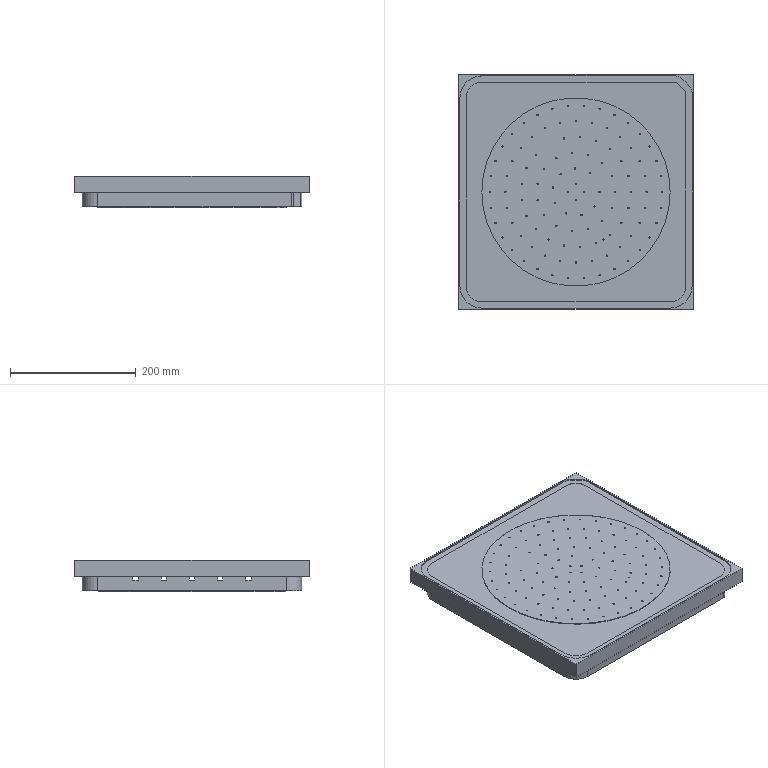NC program | NX | posted with a generic post | part box 374 x 374 x 49.5 mm
Lines 1 to 1179 of 17720:
N10 G17 G21 G94 G90
(01 , TOOL : D16R0.8)
N12 T00 M6
N14 G53
N16 G17 G0 G90 X-176.97 Y-25.521 S7000 M3 M8
N18 G43 Z105.5 H0
N20 Z26.5
N22 G94 G1 Y0. Z25.163 F4500.
N24 Y150.
N26 G2 X-150. Y176.97 R26.97
N28 G1 X157.929
N30 G2 X162.858 Y174.929 R6.97
N32 G1 X174.929 Y162.858
N34 G2 X176.97 Y157.929 R6.97
N36 G1 Y-150.
N38 G2 X150. Y-176.97 R26.97
N40 G1 X-150.
N42 G2 X-176.97 Y-150. R26.97
N44 G1 Y0.
N46 X-166.89
N48 Y150.
N50 G2 X-150. Y166.89 R16.89
N52 G1 X156.641
N54 X166.89 Y156.641
N56 Y-150.
N58 G2 X150. Y-166.89 R16.89
N60 G1 X-150.
N62 G2 X-166.89 Y-150. R16.89
N64 G1 Y0.
N66 X-156.81
N68 Y150.
N70 G2 X-150. Y156.81 R6.81
N72 G1 X152.466
N74 X156.81 Y152.466
N76 Y-150.
N78 G2 X150. Y-156.81 R6.81
N80 G1 X-150.
N82 G2 X-156.81 Y-150. R6.81
N84 G1 Y0.
N86 X-146.73
N88 Y146.73
N90 X146.73
N92 Y-146.73
N94 X-146.73
N96 Y0.
N98 X-136.65
N100 Y136.65
N102 X136.65
N104 Y-136.65
N106 X-136.65
N108 Y0.
N110 X-126.57
N112 Y126.57
N114 X126.57
N116 Y-126.57
N118 X-126.57
N120 Y0.
N122 X-116.49
N124 Y116.49
N126 X116.49
N128 Y-116.49
N130 X-116.49
N132 Y0.
N134 X-106.41
N136 Y106.41
N138 X106.41
N140 Y-106.41
N142 X-106.41
N144 Y0.
N146 X-96.33
N148 Y96.33
N150 X96.33
N152 Y-96.33
N154 X-96.33
N156 Y0.
N158 X-86.25
N160 Y86.25
N162 X86.25
N164 Y-86.25
N166 X-86.25
N168 Y0.
N170 X-76.17
N172 Y76.17
N174 X76.17
N176 Y-76.17
N178 X-76.17
N180 Y0.
N182 X-66.09
N184 Y66.09
N186 X66.09
N188 Y-66.09
N190 X-66.09
N192 Y0.
N194 X-56.01
N196 Y56.01
N198 X56.01
N200 Y-56.01
N202 X-56.01
N204 Y0.
N206 X-45.93
N208 Y45.93
N210 X45.93
N212 Y-45.93
N214 X-45.93
N216 Y0.
N218 X-35.85
N220 Y35.85
N222 X35.85
N224 Y-35.85
N226 X-35.85
N228 Y0.
N230 X-25.77
N232 Y25.77
N234 X25.77
N236 Y-25.77
N238 X-25.77
N240 Y0.
N242 X-15.69
N244 Y15.69
N246 X15.69
N248 Y-15.69
N250 X-15.69
N252 Y0.
N254 X-5.61
N256 Y5.61
N258 X5.61
N260 Y-5.61
N262 X-5.61
N264 Y0.
N266 G3 X-8.81 Y3.2 R3.2
N268 G1 Z26.163
N270 G0 Z28.5
N272 X-176.858 Y-25.521
N274 Z26.163
N276 G1 Y0. Z24.825
N278 Y150.
N280 G2 X-150. Y176.858 R26.858
N282 G1 X157.929
N284 G2 X162.778 Y174.85 R6.858
N286 G1 X174.85 Y162.778
N288 G2 X176.858 Y157.929 R6.858
N290 G1 Y-150.
N292 G2 X150. Y-176.858 R26.858
N294 G1 X-150.
N296 G2 X-176.858 Y-150. R26.858
N298 G1 Y0.
N300 X-166.778
N302 Y150.
N304 G2 X-150. Y166.778 R16.778
N306 G1 X156.594
N308 X166.778 Y156.594
N310 Y-150.
N312 G2 X150. Y-166.778 R16.778
N314 G1 X-150.
N316 G2 X-166.778 Y-150. R16.778
N318 G1 Y0.
N320 X-156.698
N322 Y150.
N324 G2 X-150. Y156.698 R6.698
N326 G1 X152.419
N328 X156.698 Y152.419
N330 Y-150.
N332 G2 X150. Y-156.698 R6.698
N334 G1 X-150.
N336 G2 X-156.698 Y-150. R6.698
N338 G1 Y0.
N340 X-146.618
N342 Y146.618
N344 X146.618
N346 Y-146.618
N348 X-146.618
N350 Y0.
N352 X-136.538
N354 Y136.538
N356 X136.538
N358 Y-136.538
N360 X-136.538
N362 Y0.
N364 X-126.458
N366 Y126.458
N368 X126.458
N370 Y-126.458
N372 X-126.458
N374 Y0.
N376 X-116.378
N378 Y116.378
N380 X116.378
N382 Y-116.378
N384 X-116.378
N386 Y0.
N388 X-106.298
N390 Y106.298
N392 X106.298
N394 Y-106.298
N396 X-106.298
N398 Y0.
N400 X-96.218
N402 Y96.218
N404 X96.218
N406 Y-96.218
N408 X-96.218
N410 Y0.
N412 X-86.138
N414 Y86.138
N416 X86.138
N418 Y-86.138
N420 X-86.138
N422 Y0.
N424 X-76.058
N426 Y76.058
N428 X76.058
N430 Y-76.058
N432 X-76.058
N434 Y0.
N436 X-65.978
N438 Y65.978
N440 X65.978
N442 Y-65.978
N444 X-65.978
N446 Y0.
N448 X-55.898
N450 Y55.898
N452 X55.898
N454 Y-55.898
N456 X-55.898
N458 Y0.
N460 X-45.818
N462 Y45.818
N464 X45.818
N466 Y-45.818
N468 X-45.818
N470 Y0.
N472 X-35.738
N474 Y35.738
N476 X35.738
N478 Y-35.738
N480 X-35.738
N482 Y0.
N484 X-25.658
N486 Y25.658
N488 X25.658
N490 Y-25.658
N492 X-25.658
N494 Y0.
N496 X-15.578
N498 Y15.578
N500 X15.578
N502 Y-15.578
N504 X-15.578
N506 Y0.
N508 X-5.498
N510 Y5.498
N512 X5.498
N514 Y-5.498
N516 X-5.498
N518 Y0.
N520 G3 X-8.698 Y3.2 R3.2
N522 G1 Z25.825
N524 G0 Z28.163
N526 X-176.85 Y-25.521
N528 Z25.825
N530 G1 Y0. Z24.488
N532 Y150.
N534 G2 X-150. Y176.85 R26.85
N536 G1 X157.929
N538 G2 X162.773 Y174.844 R6.85
N540 G1 X174.844 Y162.773
N542 G2 X176.85 Y157.929 R6.85
N544 G1 Y-150.
N546 G2 X150. Y-176.85 R26.85
N548 G1 X-150.
N550 G2 X-176.85 Y-150. R26.85
N552 G1 Y0.
N554 X-166.77
N556 Y150.
N558 G2 X-150. Y166.77 R16.77
N560 G1 X156.591
N562 X166.77 Y156.591
N564 Y-150.
N566 G2 X150. Y-166.77 R16.77
N568 G1 X-150.
N570 G2 X-166.77 Y-150. R16.77
N572 G1 Y0.
N574 X-156.69
N576 Y150.
N578 G2 X-150. Y156.69 R6.69
N580 G1 X152.416
N582 X156.69 Y152.416
N584 Y-150.001
N586 G2 X150. Y-156.69 R6.69
N588 G1 X-150.
N590 G2 X-156.69 Y-150. R6.69
N592 G1 Y0.
N594 X-146.61
N596 Y146.61
N598 X146.61
N600 Y-146.61
N602 X-146.61
N604 Y0.
N606 X-136.53
N608 Y136.53
N610 X136.53
N612 Y-136.53
N614 X-136.53
N616 Y0.
N618 X-126.45
N620 Y126.45
N622 X126.45
N624 Y-126.45
N626 X-126.45
N628 Y0.
N630 X-116.37
N632 Y116.37
N634 X116.37
N636 Y-116.37
N638 X-116.37
N640 Y0.
N642 X-106.29
N644 Y106.29
N646 X106.29
N648 Y-106.29
N650 X-106.29
N652 Y0.
N654 X-96.21
N656 Y96.21
N658 X96.21
N660 Y-96.21
N662 X-96.21
N664 Y0.
N666 X-86.13
N668 Y86.13
N670 X86.13
N672 Y-86.13
N674 X-86.13
N676 Y0.
N678 X-76.05
N680 Y76.05
N682 X76.05
N684 Y-76.05
N686 X-76.05
N688 Y0.
N690 X-65.97
N692 Y65.97
N694 X65.97
N696 Y-65.97
N698 X-65.97
N700 Y0.
N702 X-55.89
N704 Y55.89
N706 X55.89
N708 Y-55.89
N710 X-55.89
N712 Y0.
N714 X-45.81
N716 Y45.81
N718 X45.81
N720 Y-45.81
N722 X-45.81
N724 Y0.
N726 X-35.73
N728 Y35.73
N730 X35.73
N732 Y-35.73
N734 X-35.73
N736 Y0.
N738 X-25.65
N740 Y25.65
N742 X25.65
N744 Y-25.65
N746 X-25.65
N748 Y0.
N750 X-15.57
N752 Y15.57
N754 X15.57
N756 Y-15.57
N758 X-15.57
N760 Y0.
N762 X-5.49
N764 Y5.49
N766 X5.49
N768 Y-5.49
N770 X-5.49
N772 Y0.
N774 G3 X-8.69 Y3.2 R3.2
N776 G1 Z25.488
N778 G0 Z27.825
N780 X-176.85 Y-25.521
N782 Z25.488
N784 G1 Y0. Z24.15
N786 Y150.
N788 G2 X-150. Y176.85 R26.85
N790 G1 X157.929
N792 G2 X162.773 Y174.844 R6.85
N794 G1 X174.844 Y162.773
N796 G2 X176.85 Y157.929 R6.85
N798 G1 Y-150.
N800 G2 X150. Y-176.85 R26.85
N802 G1 X-150.
N804 G2 X-176.85 Y-150. R26.85
N806 G1 Y0.
N808 X-166.77
N810 Y150.
N812 G2 X-150. Y166.77 R16.77
N814 G1 X156.591
N816 X166.77 Y156.591
N818 Y-150.
N820 G2 X150. Y-166.77 R16.77
N822 G1 X-150.
N824 G2 X-166.77 Y-150. R16.77
N826 G1 Y0.
N828 X-156.69
N830 Y150.
N832 G2 X-150. Y156.69 R6.69
N834 G1 X152.416
N836 X156.69 Y152.416
N838 Y-150.001
N840 G2 X150. Y-156.69 R6.69
N842 G1 X-150.
N844 G2 X-156.69 Y-150. R6.69
N846 G1 Y0.
N848 X-146.61
N850 Y146.61
N852 X146.61
N854 Y-146.61
N856 X-146.61
N858 Y0.
N860 X-136.53
N862 Y136.53
N864 X136.53
N866 Y-136.53
N868 X-136.53
N870 Y0.
N872 X-126.45
N874 Y126.45
N876 X126.45
N878 Y-126.45
N880 X-126.45
N882 Y0.
N884 X-116.37
N886 Y116.37
N888 X116.37
N890 Y-116.37
N892 X-116.37
N894 Y0.
N896 X-106.29
N898 Y106.29
N900 X106.29
N902 Y-106.29
N904 X-106.29
N906 Y0.
N908 X-96.21
N910 Y96.21
N912 X96.21
N914 Y-96.21
N916 X-96.21
N918 Y0.
N920 X-86.13
N922 Y86.13
N924 X86.13
N926 Y-86.13
N928 X-86.13
N930 Y0.
N932 X-76.05
N934 Y76.05
N936 X76.05
N938 Y-76.05
N940 X-76.05
N942 Y0.
N944 X-65.97
N946 Y65.97
N948 X65.97
N950 Y-65.97
N952 X-65.97
N954 Y0.
N956 X-55.89
N958 Y55.89
N960 X55.89
N962 Y-55.89
N964 X-55.89
N966 Y0.
N968 X-45.81
N970 Y45.81
N972 X45.81
N974 Y-45.81
N976 X-45.81
N978 Y0.
N980 X-35.73
N982 Y35.73
N984 X35.73
N986 Y-35.73
N988 X-35.73
N990 Y0.
N992 X-25.65
N994 Y25.65
N996 X25.65
N998 Y-25.65
N1000 X-25.65
N1002 Y0.
N1004 X-15.57
N1006 Y15.57
N1008 X15.57
N1010 Y-15.57
N1012 X-15.57
N1014 Y0.
N1016 X-5.49
N1018 Y5.49
N1020 X5.49
N1022 Y-5.49
N1024 X-5.49
N1026 Y0.
N1028 G3 X-8.69 Y3.2 R3.2
N1030 G1 Z25.15
N1032 G0 Z27.488
N1034 X-176.85 Y-25.442
N1036 Z25.15
N1038 G1 Y0. Z23.817
N1040 Y150.
N1042 G2 X-150. Y176.85 R26.85
N1044 G1 X157.929
N1046 G2 X162.773 Y174.844 R6.85
N1048 G1 X174.844 Y162.773
N1050 G2 X176.85 Y157.929 R6.85
N1052 G1 Y-150.
N1054 G2 X150. Y-176.85 R26.85
N1056 G1 X-150.
N1058 G2 X-176.85 Y-150. R26.85
N1060 G1 Y0.
N1062 X-166.77
N1064 Y150.
N1066 G2 X-150. Y166.77 R16.77
N1068 G1 X-32.072
N1070 Y156.69
N1072 G3 X-156.69 Y32.072 R159.939
N1074 G1 X-159.57 Y25.473
N1076 Y10.853
N1078 G2 X-157.975 Y24.988 R159.939
N1080 X-159.57 Y25.473 R7.2
N1082 G1 X-156.69 Y32.072
N1084 Y150.
N1086 G2 X-150. Y156.69 R6.69
N1088 G1 X-86.092
N1090 Y146.61
N1092 G3 X-146.61 Y86.092 R170.019
N1094 G1 X-148.782 Y77.696
N1096 X-146.61 Y86.092
N1098 Y146.61
N1100 X-117.452
N1102 Y136.53
N1104 G3 X-136.53 Y117.452 R180.099
N1106 G1 X-139.117 Y110.261
N1108 X-136.53 Y117.452
N1110 Y136.53
N1112 X-117.452
N1114 X-110.261 Y139.117
N1116 X-117.452 Y136.53
N1118 Y146.61
N1120 X-86.092
N1122 X-77.696 Y148.782
N1124 X-86.092 Y146.61
N1126 Y156.69
N1128 X-32.072
N1130 X-24.988 Y157.975
N1132 G2 X-10.853 Y159.57 R159.939
N1134 G1 X-25.473
N1136 G2 X-24.988 Y157.975 R7.2
N1138 G1 X-32.072 Y156.69
N1140 Y166.77
N1142 X156.591
N1144 X166.77 Y156.591
N1146 Y32.072
N1148 X156.69
N1150 G3 X32.072 Y156.69 R159.939
N1152 G1 X25.473 Y159.57
N1154 X10.853
N1156 G2 X24.988 Y157.975 R159.939
N1158 X25.473 Y159.57 R7.2
N1160 G1 X32.072 Y156.69
N1162 X152.416
N1164 X156.69 Y152.416
N1166 Y86.092
N1168 X146.61
N1170 G3 X86.092 Y146.61 R170.019
N1172 G1 X77.696 Y148.782
N1174 X86.092 Y146.61
N1176 X146.61
N1178 Y117.452
N1180 X136.53
N1182 G3 X117.452 Y136.53 R180.099
N1184 G1 X110.261 Y139.117
N1186 X117.452 Y136.53
N1188 X136.53
N1190 Y117.452
N1192 X139.117 Y110.261
N1194 X136.53 Y117.452
N1196 X146.61
N1198 Y86.092
N1200 X148.782 Y77.696
N1202 X146.61 Y86.092
N1204 X156.69
N1206 Y32.072
N1208 X157.975 Y24.988
N1210 G2 X159.57 Y10.853 R159.939
N1212 G1 Y25.473
N1214 G2 X157.975 Y24.988 R7.2
N1216 G1 X156.69 Y32.072
N1218 X166.77
N1220 Y-150.
N1222 G2 X150. Y-166.77 R16.77
N1224 G1 X32.072
N1226 Y-156.69
N1228 G3 X156.69 Y-32.072 R159.939
N1230 G1 X159.57 Y-25.473
N1232 Y-10.853
N1234 G2 X157.975 Y-24.988 R159.939
N1236 X159.57 Y-25.473 R7.2
N1238 G1 X156.69 Y-32.072
N1240 Y-150.
N1242 G2 X150. Y-156.69 R6.69
N1244 G1 X86.092
N1246 Y-146.61
N1248 G3 X146.61 Y-86.092 R170.019
N1250 G1 X148.782 Y-77.696
N1252 X146.61 Y-86.092
N1254 Y-146.61
N1256 X117.452
N1258 Y-136.53
N1260 G3 X136.53 Y-117.452 R180.099
N1262 G1 X139.117 Y-110.261
N1264 X136.53 Y-117.452
N1266 Y-136.53
N1268 X117.452
N1270 X110.261 Y-139.117
N1272 X117.452 Y-136.53
N1274 Y-146.61
N1276 X86.092
N1278 X77.696 Y-148.782
N1280 X86.092 Y-146.61
N1282 Y-156.69
N1284 X32.072
N1286 X24.988 Y-157.975
N1288 G2 X10.853 Y-159.57 R159.939
N1290 G1 X25.473
N1292 G2 X24.988 Y-157.975 R7.2
N1294 G1 X32.072 Y-156.69
N1296 Y-166.77
N1298 X-150.
N1300 G2 X-166.77 Y-150. R16.77
N1302 G1 Y-32.072
N1304 X-156.69
N1306 G3 X-32.072 Y-156.69 R159.939
N1308 G1 X-25.473 Y-159.57
N1310 X-10.853
N1312 G2 X-24.988 Y-157.975 R159.939
N1314 X-25.473 Y-159.57 R7.2
N1316 G1 X-32.072 Y-156.69
N1318 X-31.668 Y-154.715
N1320 G2 X-154.715 Y31.668 R157.923
N1322 X-31.668 Y-154.715 R-157.923
N1324 G1 X-32.072 Y-156.69
N1326 X-150.
N1328 G2 X-156.69 Y-150. R6.69
N1330 G1 Y-86.092
N1332 X-146.61
N1334 G3 X-86.092 Y-146.61 R170.019
N1336 G1 X-77.696 Y-148.782
N1338 X-86.092 Y-146.61
N1340 X-146.61
N1342 Y-117.452
N1344 X-136.53
N1346 G3 X-117.452 Y-136.53 R180.099
N1348 G1 X-110.261 Y-139.117
N1350 X-117.452 Y-136.53
N1352 X-136.53
N1354 Y-117.452
N1356 X-139.117 Y-110.261
N1358 X-136.53 Y-117.452
N1360 X-146.61
N1362 Y-86.092
N1364 X-148.782 Y-77.696
N1366 X-146.61 Y-86.092
N1368 X-156.69
N1370 Y-32.072
N1372 X-157.975 Y-24.988
N1374 G2 X-159.57 Y-10.853 R159.939
N1376 G1 Y-25.473
N1378 G2 X-157.975 Y-24.988 R7.2
N1380 G1 X-156.69 Y-32.072
N1382 X-166.77
N1384 Y0.
N1386 G3 X-169.97 Y3.2 R3.2
N1388 G1 Z24.817
N1390 G0 Z27.15
N1392 X-176.85 Y-25.442
N1394 Z24.817
N1396 G1 Y0. Z23.483
N1398 Y150.
N1400 G2 X-150. Y176.85 R26.85
N1402 G1 X157.929
N1404 G2 X162.773 Y174.844 R6.85
N1406 G1 X174.844 Y162.773
N1408 G2 X176.85 Y157.929 R6.85
N1410 G1 Y-150.
N1412 G2 X150. Y-176.85 R26.85
N1414 G1 X-150.
N1416 G2 X-176.85 Y-150. R26.85
N1418 G1 Y0.
N1420 X-166.77
N1422 Y150.
N1424 G2 X-150. Y166.77 R16.77
N1426 G1 X-32.978
N1428 Y156.69
N1430 G3 X-156.69 Y32.978 R160.123
N1432 G1 X-159.57 Y26.379
N1434 Y13.293
N1436 G2 X-158.014 Y25.901 R160.123
N1438 X-159.57 Y26.379 R7.2
N1440 G1 X-156.69 Y32.978
N1442 Y150.
N1444 G2 X-150. Y156.69 R6.69
N1446 G1 X-86.455
N1448 Y146.61
N1450 G3 X-146.61 Y86.455 R170.203
N1452 G1 X-148.787 Y78.076
N1454 X-146.61 Y86.455
N1456 Y146.61
N1458 X-117.735
N1460 Y136.53
N1462 G3 X-136.53 Y117.735 R180.283
N1464 G1 X-139.12 Y110.549
N1466 X-136.53 Y117.735
N1468 Y136.53
N1470 X-117.735
N1472 X-110.549 Y139.12
N1474 X-117.735 Y136.53
N1476 Y146.61
N1478 X-86.455
N1480 X-78.076 Y148.787
N1482 X-86.455 Y146.61
N1484 Y156.69
N1486 X-32.978
N1488 X-25.901 Y158.014
N1490 G2 X-13.293 Y159.57 R160.123
N1492 G1 X-26.379
N1494 G2 X-25.901 Y158.014 R7.2
N1496 G1 X-32.978 Y156.69
N1498 Y166.77
N1500 X156.591
N1502 X166.77 Y156.591
N1504 Y32.978
N1506 X156.69
N1508 G3 X32.978 Y156.69 R160.123
N1510 G1 X26.379 Y159.57
N1512 X13.293
N1514 G2 X25.901 Y158.014 R160.123
N1516 X26.379 Y159.57 R7.2
N1518 G1 X32.978 Y156.69
N1520 X152.416
N1522 X156.69 Y152.416
N1524 Y86.455
N1526 X146.61
N1528 G3 X86.455 Y146.61 R170.203
N1530 G1 X78.076 Y148.787
N1532 X86.455 Y146.61
N1534 X146.61
N1536 Y117.735
N1538 X136.53
N1540 G3 X117.735 Y136.53 R180.283
N1542 G1 X110.549 Y139.12
N1544 X117.735 Y136.53
N1546 X136.53
N1548 Y117.735
N1550 X139.12 Y110.549
N1552 X136.53 Y117.735
N1554 X146.61
N1556 Y86.455
N1558 X148.787 Y78.076
N1560 X146.61 Y86.455
N1562 X156.69
N1564 Y32.978
N1566 X158.014 Y25.901
N1568 G2 X159.57 Y13.293 R160.123
N1570 G1 Y26.379
N1572 G2 X158.014 Y25.901 R7.2
N1574 G1 X156.69 Y32.978
N1576 X166.77
N1578 Y-150.
N1580 G2 X150. Y-166.77 R16.77
N1582 G1 X32.978
N1584 Y-156.69
N1586 G3 X156.69 Y-32.978 R160.123
N1588 G1 X159.57 Y-26.379
N1590 Y-13.293
N1592 G2 X158.014 Y-25.901 R160.123
N1594 X159.57 Y-26.379 R7.2
N1596 G1 X156.69 Y-32.978
N1598 Y-150.
N1600 G2 X150. Y-156.69 R6.69
N1602 G1 X86.455
N1604 Y-146.61
N1606 G3 X146.61 Y-86.455 R170.203
N1608 G1 X148.787 Y-78.076
N1610 X146.61 Y-86.455
N1612 Y-146.61
N1614 X117.735
N1616 Y-136.53
N1618 G3 X136.53 Y-117.735 R180.283
N1620 G1 X139.12 Y-110.549
N1622 X136.53 Y-117.735
N1624 Y-136.53
N1626 X117.735
N1628 X110.549 Y-139.12
N1630 X117.735 Y-136.53
N1632 Y-146.61
N1634 X86.455
N1636 X78.076 Y-148.787
N1638 X86.455 Y-146.61
N1640 Y-156.69
N1642 X32.978
N1644 X25.901 Y-158.014
N1646 G2 X13.293 Y-159.57 R160.123
N1648 G1 X26.379
N1650 G2 X25.901 Y-158.014 R7.2
N1652 G1 X32.978 Y-156.69
N1654 Y-166.77
N1656 X-150.
N1658 G2 X-166.77 Y-150. R16.77
N1660 G1 Y-32.978
N1662 X-156.69
N1664 G3 X-32.978 Y-156.69 R160.123
N1666 G1 X-26.379 Y-159.57
N1668 X-13.293
N1670 G2 X-25.901 Y-158.014 R160.123
N1672 X-26.379 Y-159.57 R7.2
N1674 G1 X-32.978 Y-156.69
N1676 X-32.563 Y-154.717
N1678 G2 X-154.717 Y32.563 R158.107
N1680 X-32.563 Y-154.717 R-158.107
N1682 G1 X-32.978 Y-156.69
N1684 X-150.
N1686 G2 X-156.69 Y-150. R6.69
N1688 G1 Y-86.455
N1690 X-146.61
N1692 G3 X-86.455 Y-146.61 R170.203
N1694 G1 X-78.076 Y-148.787
N1696 X-86.455 Y-146.61
N1698 X-146.61
N1700 Y-117.735
N1702 X-136.53
N1704 G3 X-117.735 Y-136.53 R180.283
N1706 G1 X-110.549 Y-139.12
N1708 X-117.735 Y-136.53
N1710 X-136.53
N1712 Y-117.735
N1714 X-139.12 Y-110.549
N1716 X-136.53 Y-117.735
N1718 X-146.61
N1720 Y-86.455
N1722 X-148.787 Y-78.076
N1724 X-146.61 Y-86.455
N1726 X-156.69
N1728 Y-32.978
N1730 X-158.014 Y-25.901
N1732 G2 X-159.57 Y-13.293 R160.123
N1734 G1 Y-26.379
N1736 G2 X-158.014 Y-25.901 R7.2
N1738 G1 X-156.69 Y-32.978
N1740 X-166.77
N1742 Y0.
N1744 G3 X-169.97 Y3.2 R3.2
N1746 G1 Z24.483
N1748 G0 Z26.817
N1750 X-176.85 Y-25.442
N1752 Z24.483
N1754 G1 Y0. Z23.15
N1756 Y150.
N1758 G2 X-150. Y176.85 R26.85
N1760 G1 X157.929
N1762 G2 X162.773 Y174.844 R6.85
N1764 G1 X174.844 Y162.773
N1766 G2 X176.85 Y157.929 R6.85
N1768 G1 Y-150.
N1770 G2 X150. Y-176.85 R26.85
N1772 G1 X-150.
N1774 G2 X-176.85 Y-150. R26.85
N1776 G1 Y0.
N1778 X-166.77
N1780 Y150.
N1782 G2 X-150. Y166.77 R16.77
N1784 G1 X-33.187
N1786 Y156.69
N1788 G3 X-156.69 Y33.187 R160.166
N1790 G1 X-159.57 Y26.588
N1792 Y13.804
N1794 G2 X-158.023 Y26.112 R160.166
N1796 X-159.57 Y26.588 R7.2
N1798 G1 X-156.69 Y33.187
N1800 Y150.
N1802 G2 X-150. Y156.69 R6.69
N1804 G1 X-86.54
N1806 Y146.61
N1808 G3 X-146.61 Y86.54 R170.246
N1810 G1 X-148.788 Y78.164
N1812 X-146.61 Y86.54
N1814 Y146.61
N1816 X-117.801
N1818 Y136.53
N1820 G3 X-136.53 Y117.801 R180.326
N1822 G1 X-139.12 Y110.617
N1824 X-136.53 Y117.801
N1826 Y136.53
N1828 X-117.801
N1830 X-110.617 Y139.12
N1832 X-117.801 Y136.53
N1834 Y146.61
N1836 X-86.54
N1838 X-78.164 Y148.788
N1840 X-86.54 Y146.61
N1842 Y156.69
N1844 X-33.187
N1846 X-26.112 Y158.023
N1848 G2 X-16.346 Y159.33 R160.166
N1850 X-13.804 Y159.57 R160.166
N1852 G1 X-26.588
N1854 G2 X-26.112 Y158.023 R7.2
N1856 G1 X-33.187 Y156.69
N1858 Y166.77
N1860 X156.591
N1862 X166.77 Y156.591
N1864 Y33.187
N1866 X156.69
N1868 G3 X33.187 Y156.69 R160.166
N1870 G1 X26.588 Y159.57
N1872 X13.804
N1874 G2 X26.112 Y158.023 R160.166
N1876 X26.588 Y159.57 R7.2
N1878 G1 X33.187 Y156.69
N1880 X152.416
N1882 X156.69 Y152.416
N1884 Y86.54
N1886 X146.61
N1888 G3 X86.54 Y146.61 R170.246
N1890 G1 X78.164 Y148.788
N1892 X86.54 Y146.61
N1894 X146.61
N1896 Y117.801
N1898 X136.53
N1900 G3 X117.801 Y136.53 R180.326
N1902 G1 X110.617 Y139.12
N1904 X117.801 Y136.53
N1906 X136.53
N1908 Y117.801
N1910 X139.12 Y110.617
N1912 X136.53 Y117.801
N1914 X146.61
N1916 Y86.54
N1918 X148.788 Y78.164
N1920 X146.61 Y86.54
N1922 X156.69
N1924 Y33.187
N1926 X158.023 Y26.112
N1928 G2 X159.57 Y13.804 R160.166
N1930 G1 Y26.588
N1932 G2 X158.023 Y26.112 R7.2
N1934 G1 X156.69 Y33.187
N1936 X166.77
N1938 Y-150.
N1940 G2 X150. Y-166.77 R16.77
N1942 G1 X33.187
N1944 Y-156.69
N1946 G3 X156.69 Y-33.187 R160.166
N1948 G1 X159.57 Y-26.588
N1950 Y-13.804
N1952 G2 X158.023 Y-26.112 R160.166
N1954 X159.57 Y-26.588 R7.2
N1956 G1 X156.69 Y-33.187
N1958 Y-150.001
N1960 G2 X150. Y-156.69 R6.69
N1962 G1 X86.54
N1964 Y-146.61
N1966 G3 X146.61 Y-86.54 R170.246
N1968 G1 X148.788 Y-78.164
N1970 X146.61 Y-86.54
N1972 Y-146.61
N1974 X117.801
N1976 Y-136.53
N1978 G3 X136.53 Y-117.801 R180.326
N1980 G1 X139.12 Y-110.617
N1982 X136.53 Y-117.801
N1984 Y-136.53
N1986 X117.801
N1988 X110.617 Y-139.12
N1990 X117.801 Y-136.53
N1992 Y-146.61
N1994 X86.54
N1996 X78.164 Y-148.788
N1998 X86.54 Y-146.61
N2000 Y-156.69
N2002 X33.187
N2004 X26.112 Y-158.023
N2006 G2 X13.804 Y-159.57 R160.166
N2008 G1 X26.588
N2010 G2 X26.112 Y-158.023 R7.2
N2012 G1 X33.187 Y-156.69
N2014 Y-166.77
N2016 X-150.
N2018 G2 X-166.77 Y-150. R16.77
N2020 G1 Y-33.187
N2022 X-156.69
N2024 G3 X-33.187 Y-156.69 R160.166
N2026 G1 X-26.588 Y-159.57
N2028 X-13.804
N2030 G2 X-26.112 Y-158.023 R160.166
N2032 X-26.588 Y-159.57 R7.2
N2034 G1 X-33.187 Y-156.69
N2036 X-32.769 Y-154.718
N2038 G2 X-154.718 Y32.769 R158.15
N2040 X-32.769 Y-154.718 R-158.15
N2042 G1 X-33.187 Y-156.69
N2044 X-150.
N2046 G2 X-156.69 Y-150. R6.69
N2048 G1 Y-86.54
N2050 X-146.61
N2052 G3 X-86.54 Y-146.61 R170.246
N2054 G1 X-78.164 Y-148.788
N2056 X-86.54 Y-146.61
N2058 X-146.61
N2060 Y-117.801
N2062 X-136.53
N2064 G3 X-117.801 Y-136.53 R180.326
N2066 G1 X-110.617 Y-139.12
N2068 X-117.801 Y-136.53
N2070 X-136.53
N2072 Y-117.801
N2074 X-139.12 Y-110.617
N2076 X-136.53 Y-117.801
N2078 X-146.61
N2080 Y-86.54
N2082 X-148.788 Y-78.164
N2084 X-146.61 Y-86.54
N2086 X-156.69
N2088 Y-33.187
N2090 X-158.023 Y-26.112
N2092 G2 X-159.57 Y-13.804 R160.166
N2094 G1 Y-26.588
N2096 G2 X-158.023 Y-26.112 R7.2
N2098 G1 X-156.69 Y-33.187
N2100 X-166.77
N2102 Y0.
N2104 G3 X-169.97 Y3.2 R3.2
N2106 G1 Z24.15
N2108 G0 Z105.5
N2110 M9
N2112 M5
(02 , TOOL : V2.0)
N2114 M6
N2116 G53
N2118 G17 G0 G90 X-64.142 Y59.515 S2000 M3 M8
N2120 G43 Z105.5 H0
N2122 G94 G81 G98 Z22. F150. R27.
N2124 X-78.835 Y37.965
N2126 X-101.359 Y48.812
N2128 X-87.956 Y70.143
N2130 X-70.143 Y87.956
N2132 X-48.812 Y101.359
N2134 X-25.034 Y109.679
N2136 X-19.471 Y85.306
N2138 X6.539 Y87.255
N2140 X0. Y112.5
N2142 X25.034 Y109.679
N2144 X48.812 Y101.359
N2146 X61.289 Y123.085
N2148 X37.629 Y132.251
N2150 X12.687 Y136.913
N2152 X-12.687
N2154 X-37.629 Y132.251
N2156 X-61.289 Y123.085
N2158 X-82.862 Y109.727
N2160 X-101.614 Y92.633
N2162 X-116.905 Y72.384
N2164 X-128.215 Y49.671
N2166 X-135.159 Y25.266
N2168 X-109.679 Y25.034
N2170 X-112.5 Y0.
N2172 X-137.5
N2174 X-135.159 Y-25.266
N2176 X-128.215 Y-49.671
N2178 X-116.905 Y-72.384
N2180 X-101.614 Y-92.633
N2182 X-82.862 Y-109.727
N2184 X-70.143 Y-87.956
N2186 X-87.956 Y-70.143
N2188 X-64.142 Y-59.515
N2190 X-43.75 Y-75.777
N2192 X-48.812 Y-101.359
N2194 X-61.289 Y-123.085
N2196 X-37.629 Y-132.251
N2198 X-12.687 Y-136.913
N2200 X-25.034 Y-109.679
N2202 X-19.471 Y-85.306
N2204 X-6.533 Y-62.158
N2206 X19.314 Y-59.441
N2208 X8.821 Y-36.448
N2210 X0. Y-12.5
N2212 X-12.5 Y0.
N2214 X0. Y12.5
N2216 X12.5 Y0.
N2218 X37.5
N2220 X29.471 Y-23.189
N2222 X41.821 Y-46.447
N2224 X54.555 Y-68.41
N2226 X43.75 Y-75.777
N2228 X31.967 Y-81.451
N2230 X6.539 Y-87.255
N2232 X0. Y-112.5
N2234 X12.687 Y-136.913
N2236 X37.629 Y-132.251
N2238 X25.034 Y-109.679
N2240 X48.812 Y-101.359
N2242 X61.289 Y-123.085
N2244 X82.862 Y-109.727
N2246 X101.614 Y-92.633
N2248 X70.143 Y-87.956
N2250 X87.956 Y-70.143
N2252 X72.296 Y-49.291
N2254 X57.097 Y-25.421
N2256 X83.613 Y-25.791
N2258 X109.679 Y-25.034
N2260 X101.359 Y-48.812
N2262 X116.905 Y-72.384
N2264 X128.215 Y-49.671
N2266 X135.159 Y-25.266
N2268 X137.5 Y0.
N2270 X112.5
N2272 X87.5
N2274 X62.5
N2276 X57.097 Y25.421
N2278 X41.821 Y46.447
N2280 X21.818 Y30.5
N2282 X-1.714 Y37.461
N2284 X-24.512 Y28.38
N2286 X-36.813 Y7.146
N2288 X-33.35 Y-17.148
N2290 X-15.606 Y-34.099
N2292 X-31.25 Y-54.127
N2294 X-50.564 Y-36.737
N2296 X-61.134 Y-12.994
N2298 X-78.835 Y-37.965
N2300 X-101.359 Y-48.812
N2302 X-109.679 Y-25.034
N2304 X-86.523 Y-13.041
N2306 Y13.041
N2308 X-61.134 Y12.994
N2310 X-50.564 Y36.737
N2312 X-31.25 Y54.127
N2314 X-6.533 Y62.158
N2316 X19.314 Y59.441
N2318 X31.967 Y81.451
N2320 X54.555 Y68.41
N2322 X70.143 Y87.956
N2324 X82.862 Y109.727
N2326 X101.614 Y92.633
N2328 X116.905 Y72.384
N2330 X128.215 Y49.671
N2332 X135.159 Y25.266
N2334 X109.679 Y25.034
N2336 X101.359 Y48.812
N2338 X87.956 Y70.143
N2340 X72.296 Y49.291
N2342 X83.613 Y25.791
N2344 G80
N2346 G0 X83.613 Y25.791 Z105.5
N2348 M9
N2350 M5